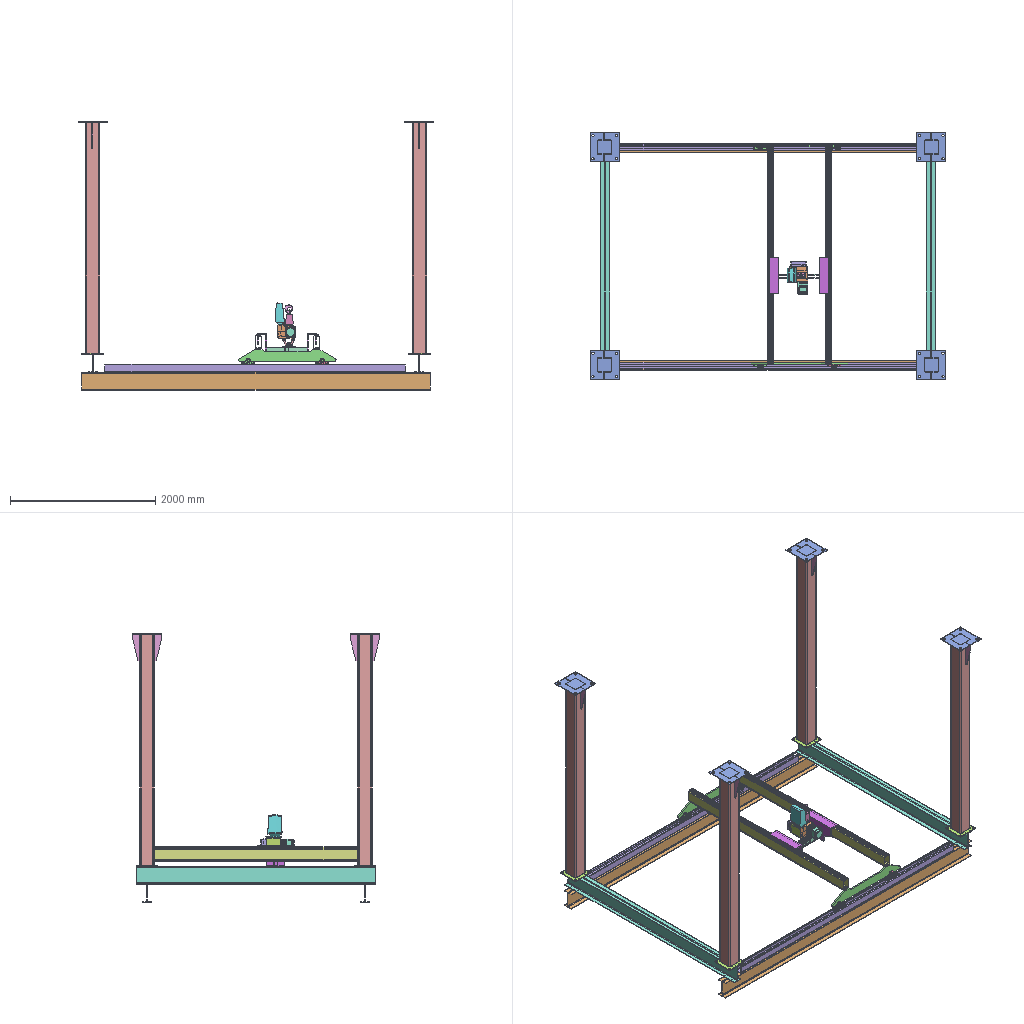Assembly | SolidWorks | 29 different items | 56 placed | box 4900 x 3400 x 3700 mm
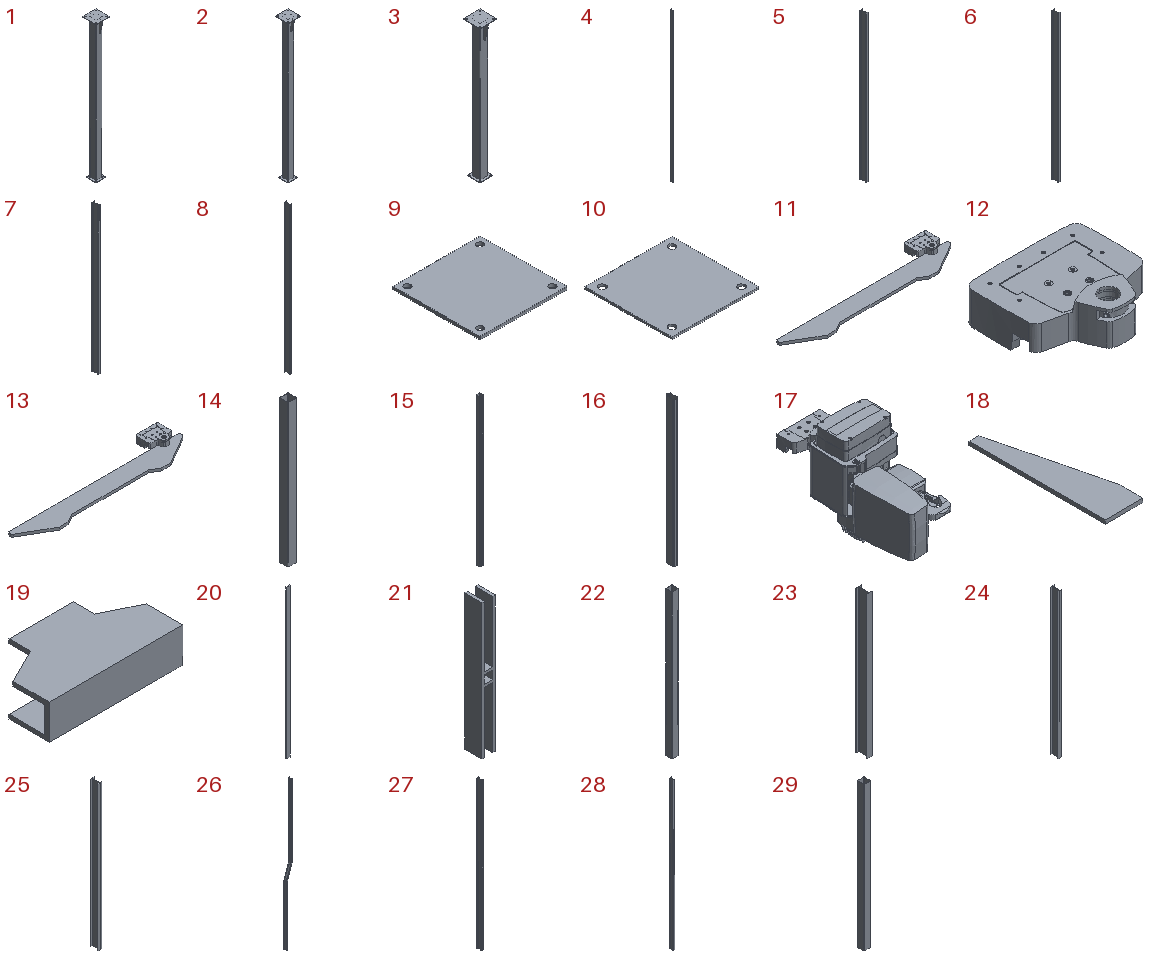Parts list (item | name | quantity | parent item | size | volume | features):
1 | (subassembly) | x1 | - | 400 x 400 x 4200 mm | 18624700 mm3 | -
2 | (subassembly) | x1 | - | 400 x 400 x 4500 mm | 29491255 mm3 | -
3 | (subassembly) | x4 | - | 400 x 400 x 3200 mm | 21789733 mm3 | -
4 | - | x1 | - | 150 x 300 x 20067 mm | 93874848 mm3 | features Extrusion 1
5 | - | x1 | - | 150 x 300 x 8090 mm | 37845593 mm3 | features Extrusion 1
6 | - | x1 | - | 150 x 300 x 8060 mm | 37705251 mm3 | features Extrusion 1
7 | - | x1 | - | 150 x 300 x 8210 mm | 38406962 mm3 | features Extrusion 1
8 | - | x1 | - | 150 x 300 x 9710 mm | 45424068 mm3 | features Extrusion 1
9 | - | x4 | in 3 | 300 x 300 x 10 mm | 884795 mm3 | features Extrusion 1
10 | - | x4 | in 3 | 400 x 400 x 10 mm | 1567830 mm3 | features Extrusion 1
11 | - | x1 | - | 1341 x 293.909 x 70 mm | 4218452 mm3 | features BaseBody 1, Fillet 1, ICE 1, Scale 1
12 | - | x2 | - | 178.17 x 167.027 x 70 mm | 882482 mm3 | features BaseBody 1, Scale 1
13 | - | x2 | - | 1341 x 293.909 x 70 mm | 4218452 mm3 | features BaseBody 1, Fillet 1, ICE 1, Scale 1
14 | - | x4 | in 3 | 200 x 200 x 3180 mm | 18839108 mm3 | features Extrusion 1
15 | - | x2 | - | 100 x 110 x 4135 mm | 4470850 mm3 | features Extrusion 1
16 | - | x2 | - | 90 x 203.757 x 3017 mm | 5182605 mm3 | features Extrusion 1
17 | - | x1 | - | 284.321 x 680.473 x 459.6 mm | 19540266 mm3 | features BaseBody 17, ICE 1, Scale 1
18 | - | x8 | in 3 | 100 x 360 x 10 mm | 249000 mm3 | features Extrusion 1
19 | - | x2 | - | 500 x 280 x 130 mm | 3757451 mm3 | features ICE 2, Extrusion 1
20 | - | x2 | - | 70 x 14 x 3017 mm | 2956807 mm3 | features Extrusion 1
21 | - | x1 | - | 55 x 71 x 556 mm | 839220 mm3 | features ICE 2, Extrusion 1
22 | - | x1 | - | 200 x 200 x 4480 mm | 26540630 mm3 | features Extrusion 1
23 | - | x2 | - | 125 x 250 x 3300 mm | 12199896 mm3 | features Extrusion 1
24 | - | x2 | - | 125 x 250 x 4800 mm | 17745303 mm3 | features Extrusion 1
25 | - | x1 | - | 125 x 250 x 4570 mm | 16895007 mm3 | features Extrusion 1
26 | - | x1 | - | 622 x 280 x 16285 mm | 87987824 mm3 | features Sweep 1
27 | - | x1 | - | 150 x 300 x 10687 mm | 49994543 mm3 | features Extrusion 1
28 | - | x1 | - | 150 x 300 x 11647 mm | 54485491 mm3 | features Extrusion 1
29 | - | x1 | - | 200 x 200 x 4180 mm | 15674075 mm3 | features Extrusion 1
Mates (type | each side: item.copy, entity, surface, feature):
In the top assembly
Coincident | 10.1 face plane Boss-Extrude1 | 10.2 face plane Boss-Extrude1 | 2 times
Coincident | 10.3 face plane Boss-Extrude1 | 10.1 face plane Boss-Extrude1 | 2 times
Coincident | 10.4 face plane Boss-Extrude1 | 10.3 face plane Boss-Extrude1 | 2 times
Coincident | 10.4 face plane Boss-Extrude1 | 10.2 face plane Boss-Extrude1
DistanceDim | 10.2 face plane Boss-Extrude1 | 10.4 face plane Boss-Extrude1
DistanceDim | 10.4 face plane Boss-Extrude1 | 10.3 face plane Boss-Extrude1
Coincident | 9.1 face plane Boss-Extrude1 | 23.1 face plane Boss-Extrude1 | 2 times
DistanceDim | 23.1 face plane Boss-Extrude1 | 9.1 face plane Boss-Extrude1
Coincident | 9.2 face plane Boss-Extrude1 | 23.2 face plane Boss-Extrude1 | 2 times
DistanceDim | 23.2 face plane Boss-Extrude1 | 9.2 face plane Boss-Extrude1
Coincident | 23.2 face plane Boss-Extrude1 | 24.1 face plane Boss-Extrude1
Coincident | 23.2 face plane Boss-Extrude1 | 24.2 face plane Boss-Extrude1
Coincident | 9.2 edge | 24.1 face plane Boss-Extrude1
Coincident | 9.3 face plane Boss-Extrude1 | 24.2 face plane Boss-Extrude1
DistanceDim | 24.1 face plane Boss-Extrude1 | 24.2 face plane Boss-Extrude1
DistanceDim | 24.1 face plane Boss-Extrude1 | 9.2 face plane Boss-Extrude1
Coincident | 24.1 face plane Boss-Extrude1 | 15.1 face plane Boss-Extrude1
DistanceDim | 15.1 face plane Boss-Extrude1 | 24.1 face plane Boss-Extrude1
DistanceDim | 15.1 face plane Boss-Extrude1 | 23.1 face plane Boss-Extrude1
Coincident | 13.1 face plane Seitenschild-RU22_34-1-solid1 | 12.1 face plane Seitenschild-RU22_34-1-solid1 | 2 times
DistanceDim | 12.1 edge | 13.1 edge
DistanceDim | 13.1 face plane Boss-Extrude1 | 15.1 face plane Boss-Extrude1 | 2 times
Coincident | 13.2 face plane Boss-Extrude1 | 20.1 face plane Boss-Extrude1 | 2 times
Coincident | 13.2 edge | 20.1 face plane Boss-Extrude1
Coincident | 13.2 face plane Boss-Extrude1 | 20.2 face plane Boss-Extrude1 | 2 times
Coincident | 13.2 edge | 20.2 face plane Boss-Extrude1
Coincident | 20.1 face plane Boss-Extrude1 | 16.1 face plane Boss-Extrude1 | 2 times
DistanceDim | 16.1 face plane Boss-Extrude1 | 20.1 face plane Boss-Extrude1
Coincident | 20.2 face plane Boss-Extrude1 | 16.2 face plane Boss-Extrude1
Coincident | 13.2 face plane Boss-Extrude1 | 16.2 face plane Boss-Extrude1
DistanceDim | 16.2 face plane Boss-Extrude1 | 20.2 face plane Boss-Extrude1
DistanceDim | 19.1 face plane Boss-Extrude3 | 16.1 face plane Boss-Extrude1
Coincident | 16.1 face plane Boss-Extrude1 | 19.1 face plane Boss-Extrude2
Coincident | 19.1 face plane Boss-Extrude1 | 19.2 face plane Boss-Extrude1 | 2 times
Coincident | 16.2 face plane Boss-Extrude1 | 19.2 face plane Boss-Extrude3
Coincident | 19.1 face plane Boss-Extrude1 | 21.1 face plane Boss-Extrude3
DistanceDim | 21.1 face plane Boss-Extrude1 | 19.1 face plane Boss-Extrude1
DistanceDim | 21.1 face plane Boss-Extrude3 | 19.1 face plane Boss-Extrude1
Coincident | 21.1 face plane Boss-Extrude1 | 17.1 face plane Seitenschild-RU22_34-1-solid1
DistanceDim | 17.1 vertex | 10.3 face plane Boss-Extrude1
Parallel | 21.1 face plane Boss-Extrude1 | 17.1 face plane Cut-Extrude1
In subassembly 3
Coincident | 14.1 face plane Boss-Extrude1 | 10.5 face plane Boss-Extrude1
DistanceDim | 14.1 face plane Boss-Extrude1 | 10.5 face plane Boss-Extrude1 | 2 times
Coincident | 14.1 face plane Boss-Extrude1 | 9.4 face plane Boss-Extrude1
DistanceDim | 9.4 face plane Boss-Extrude1 | 14.1 face plane Boss-Extrude1 | 2 times
Coincident | 10.5 face plane Boss-Extrude1 | 18.1 face plane Boss-Extrude1
Coincident | 14.1 face plane Boss-Extrude1 | 18.1 face plane Boss-Extrude1
DistanceDim | 18.1 face plane Boss-Extrude1 | 10.5 face plane Boss-Extrude1
Coincident | 10.5 face plane Boss-Extrude1 | 18.2 face plane Boss-Extrude1
Coincident | 18.1 face plane Boss-Extrude1 | 18.2 face plane Boss-Extrude1
Coincident | 14.1 face plane Boss-Extrude1 | 18.2 face plane Boss-Extrude1